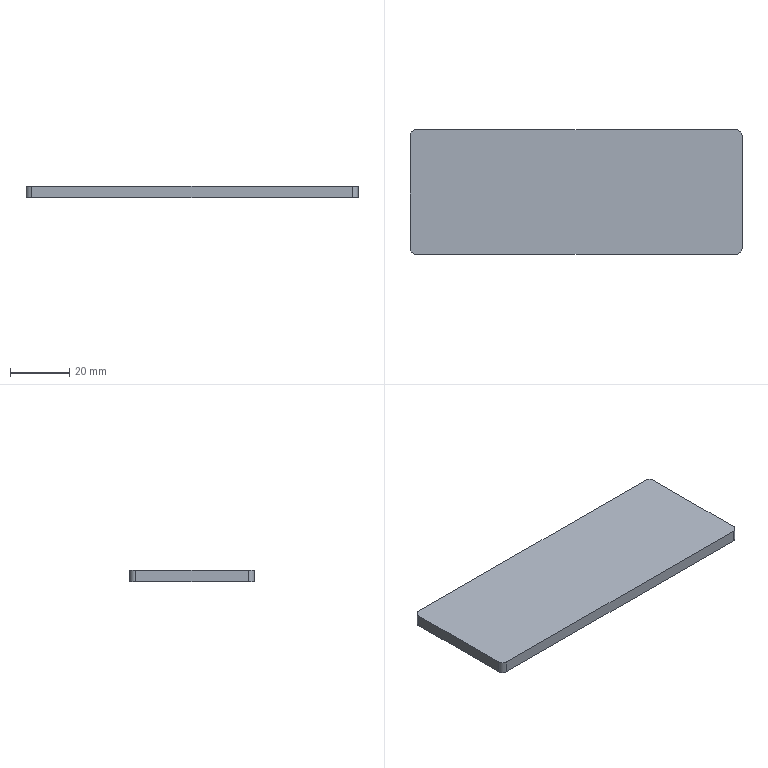Part | SolidWorks | features Extrusion 1 | 1 solid | 10 faces | box 112 x 42 x 4 mm | volume 18802 mm3 | plane 6 | cylinder 4 | commonest cylinder face diameters 4 x4
STEP:
#1=CARTESIAN_POINT('',(-54.,21.,0.));
#2=VERTEX_POINT('',#1);
#3=CARTESIAN_POINT('',(-56.,19.,0.));
#4=VERTEX_POINT('',#3);
#5=CARTESIAN_POINT('',(-54.,19.,0.));
#6=DIRECTION('',(0.,0.,1.));
#7=DIRECTION('',(1.,0.,0.));
#8=AXIS2_PLACEMENT_3D('',#5,#6,#7);
#9=CIRCLE('',#8,2.);
#10=EDGE_CURVE('',#2,#4,#9,.T.);
#11=ORIENTED_EDGE('',*,*,#10,.T.);
#12=CARTESIAN_POINT('',(-56.,19.,4.));
#13=VERTEX_POINT('',#12);
#14=CARTESIAN_POINT('',(-56.,19.,4.));
#15=DIRECTION('',(0.,0.,-1.));
#16=VECTOR('',#15,1000.);
#17=LINE('',#14,#16);
#18=EDGE_CURVE('',#13,#4,#17,.T.);
#19=ORIENTED_EDGE('',*,*,#18,.F.);
#20=CARTESIAN_POINT('',(-54.,21.,4.));
#21=VERTEX_POINT('',#20);
#22=CARTESIAN_POINT('',(-54.,19.,4.));
#23=DIRECTION('',(0.,0.,1.));
#24=DIRECTION('',(1.,0.,0.));
#25=AXIS2_PLACEMENT_3D('',#22,#23,#24);
#26=CIRCLE('',#25,2.);
#27=EDGE_CURVE('',#21,#13,#26,.T.);
#28=ORIENTED_EDGE('',*,*,#27,.F.);
#29=CARTESIAN_POINT('',(-54.,21.,4.));
#30=DIRECTION('',(0.,0.,-1.));
#31=VECTOR('',#30,1000.);
#32=LINE('',#29,#31);
#33=EDGE_CURVE('',#21,#2,#32,.T.);
#34=ORIENTED_EDGE('',*,*,#33,.T.);
#35=EDGE_LOOP('',(#11,#19,#28,#34));
#36=FACE_OUTER_BOUND('',#35,.T.);
#37=CARTESIAN_POINT('',(-54.,19.,4.));
#38=DIRECTION('',(0.,0.,-1.));
#39=DIRECTION('',(-1.,0.,0.));
#40=AXIS2_PLACEMENT_3D('',#37,#38,#39);
#41=CYLINDRICAL_SURFACE('',#40,2.);
#42=ADVANCED_FACE('',(#36),#41,.T.);
#43=CARTESIAN_POINT('',(-56.,-19.,0.));
#44=VERTEX_POINT('',#43);
#45=CARTESIAN_POINT('',(-56.,19.,0.));
#46=DIRECTION('',(0.,-1.,0.));
#47=VECTOR('',#46,1000.);
#48=LINE('',#45,#47);
#49=EDGE_CURVE('',#4,#44,#48,.T.);
#50=ORIENTED_EDGE('',*,*,#49,.T.);
#51=CARTESIAN_POINT('',(-56.,-19.,4.));
#52=VERTEX_POINT('',#51);
#53=CARTESIAN_POINT('',(-56.,-19.,4.));
#54=DIRECTION('',(0.,0.,-1.));
#55=VECTOR('',#54,1000.);
#56=LINE('',#53,#55);
#57=EDGE_CURVE('',#52,#44,#56,.T.);
#58=ORIENTED_EDGE('',*,*,#57,.F.);
#59=CARTESIAN_POINT('',(-56.,19.,4.));
#60=DIRECTION('',(0.,-1.,0.));
#61=VECTOR('',#60,1000.);
#62=LINE('',#59,#61);
#63=EDGE_CURVE('',#13,#52,#62,.T.);
#64=ORIENTED_EDGE('',*,*,#63,.F.);
#65=ORIENTED_EDGE('',*,*,#18,.T.);
#66=EDGE_LOOP('',(#50,#58,#64,#65));
#67=FACE_OUTER_BOUND('',#66,.T.);
#68=CARTESIAN_POINT('',(-56.,19.,4.));
#69=DIRECTION('',(1.,0.,0.));
#70=DIRECTION('',(0.,0.,-1.));
#71=AXIS2_PLACEMENT_3D('',#68,#69,#70);
#72=PLANE('',#71);
#73=ADVANCED_FACE('',(#67),#72,.F.);
#74=CARTESIAN_POINT('',(-54.,-21.,0.));
#75=VERTEX_POINT('',#74);
#76=CARTESIAN_POINT('',(-54.,-19.,0.));
#77=DIRECTION('',(0.,0.,-1.));
#78=DIRECTION('',(-1.,0.,0.));
#79=AXIS2_PLACEMENT_3D('',#76,#77,#78);
#80=CIRCLE('',#79,2.);
#81=EDGE_CURVE('',#75,#44,#80,.T.);
#82=ORIENTED_EDGE('',*,*,#81,.F.);
#83=CARTESIAN_POINT('',(-54.,-21.,4.));
#84=VERTEX_POINT('',#83);
#85=CARTESIAN_POINT('',(-54.,-21.,4.));
#86=DIRECTION('',(0.,0.,-1.));
#87=VECTOR('',#86,1000.);
#88=LINE('',#85,#87);
#89=EDGE_CURVE('',#84,#75,#88,.T.);
#90=ORIENTED_EDGE('',*,*,#89,.F.);
#91=CARTESIAN_POINT('',(-54.,-19.,4.));
#92=DIRECTION('',(0.,0.,-1.));
#93=DIRECTION('',(-1.,0.,0.));
#94=AXIS2_PLACEMENT_3D('',#91,#92,#93);
#95=CIRCLE('',#94,2.);
#96=EDGE_CURVE('',#84,#52,#95,.T.);
#97=ORIENTED_EDGE('',*,*,#96,.T.);
#98=ORIENTED_EDGE('',*,*,#57,.T.);
#99=EDGE_LOOP('',(#82,#90,#97,#98));
#100=FACE_OUTER_BOUND('',#99,.T.);
#101=CARTESIAN_POINT('',(-54.,-19.,4.));
#102=DIRECTION('',(0.,0.,-1.));
#103=DIRECTION('',(-1.,0.,0.));
#104=AXIS2_PLACEMENT_3D('',#101,#102,#103);
#105=CYLINDRICAL_SURFACE('',#104,2.);
#106=ADVANCED_FACE('',(#100),#105,.T.);
#107=CARTESIAN_POINT('',(54.,-21.,0.));
#108=VERTEX_POINT('',#107);
#109=CARTESIAN_POINT('',(54.,-21.,0.));
#110=DIRECTION('',(-1.,0.,0.));
#111=VECTOR('',#110,1000.);
#112=LINE('',#109,#111);
#113=EDGE_CURVE('',#108,#75,#112,.T.);
#114=ORIENTED_EDGE('',*,*,#113,.F.);
#115=CARTESIAN_POINT('',(54.,-21.,4.));
#116=VERTEX_POINT('',#115);
#117=CARTESIAN_POINT('',(54.,-21.,4.));
#118=DIRECTION('',(0.,0.,-1.));
#119=VECTOR('',#118,1000.);
#120=LINE('',#117,#119);
#121=EDGE_CURVE('',#116,#108,#120,.T.);
#122=ORIENTED_EDGE('',*,*,#121,.F.);
#123=CARTESIAN_POINT('',(54.,-21.,4.));
#124=DIRECTION('',(-1.,0.,0.));
#125=VECTOR('',#124,1000.);
#126=LINE('',#123,#125);
#127=EDGE_CURVE('',#116,#84,#126,.T.);
#128=ORIENTED_EDGE('',*,*,#127,.T.);
#129=ORIENTED_EDGE('',*,*,#89,.T.);
#130=EDGE_LOOP('',(#114,#122,#128,#129));
#131=FACE_OUTER_BOUND('',#130,.T.);
#132=CARTESIAN_POINT('',(54.,-21.,4.));
#133=DIRECTION('',(0.,-1.,0.));
#134=DIRECTION('',(1.,0.,0.));
#135=AXIS2_PLACEMENT_3D('',#132,#133,#134);
#136=PLANE('',#135);
#137=ADVANCED_FACE('',(#131),#136,.T.);
#138=CARTESIAN_POINT('',(56.,-19.,0.));
#139=VERTEX_POINT('',#138);
#140=CARTESIAN_POINT('',(54.,-19.,0.));
#141=DIRECTION('',(0.,0.,-1.));
#142=DIRECTION('',(-1.,0.,0.));
#143=AXIS2_PLACEMENT_3D('',#140,#141,#142);
#144=CIRCLE('',#143,2.);
#145=EDGE_CURVE('',#139,#108,#144,.T.);
#146=ORIENTED_EDGE('',*,*,#145,.F.);
#147=CARTESIAN_POINT('',(56.,-19.,4.));
#148=VERTEX_POINT('',#147);
#149=CARTESIAN_POINT('',(56.,-19.,4.));
#150=DIRECTION('',(0.,0.,-1.));
#151=VECTOR('',#150,1000.);
#152=LINE('',#149,#151);
#153=EDGE_CURVE('',#148,#139,#152,.T.);
#154=ORIENTED_EDGE('',*,*,#153,.F.);
#155=CARTESIAN_POINT('',(54.,-19.,4.));
#156=DIRECTION('',(0.,0.,-1.));
#157=DIRECTION('',(-1.,0.,0.));
#158=AXIS2_PLACEMENT_3D('',#155,#156,#157);
#159=CIRCLE('',#158,2.);
#160=EDGE_CURVE('',#148,#116,#159,.T.);
#161=ORIENTED_EDGE('',*,*,#160,.T.);
#162=ORIENTED_EDGE('',*,*,#121,.T.);
#163=EDGE_LOOP('',(#146,#154,#161,#162));
#164=FACE_OUTER_BOUND('',#163,.T.);
#165=CARTESIAN_POINT('',(54.,-19.,4.));
#166=DIRECTION('',(0.,0.,-1.));
#167=DIRECTION('',(-1.,0.,0.));
#168=AXIS2_PLACEMENT_3D('',#165,#166,#167);
#169=CYLINDRICAL_SURFACE('',#168,2.);
#170=ADVANCED_FACE('',(#164),#169,.T.);
#171=CARTESIAN_POINT('',(56.,19.,0.));
#172=VERTEX_POINT('',#171);
#173=CARTESIAN_POINT('',(56.,19.,0.));
#174=DIRECTION('',(0.,-1.,0.));
#175=VECTOR('',#174,1000.);
#176=LINE('',#173,#175);
#177=EDGE_CURVE('',#172,#139,#176,.T.);
#178=ORIENTED_EDGE('',*,*,#177,.F.);
#179=CARTESIAN_POINT('',(56.,19.,4.));
#180=VERTEX_POINT('',#179);
#181=CARTESIAN_POINT('',(56.,19.,4.));
#182=DIRECTION('',(0.,0.,-1.));
#183=VECTOR('',#182,1000.);
#184=LINE('',#181,#183);
#185=EDGE_CURVE('',#180,#172,#184,.T.);
#186=ORIENTED_EDGE('',*,*,#185,.F.);
#187=CARTESIAN_POINT('',(56.,19.,4.));
#188=DIRECTION('',(0.,-1.,0.));
#189=VECTOR('',#188,1000.);
#190=LINE('',#187,#189);
#191=EDGE_CURVE('',#180,#148,#190,.T.);
#192=ORIENTED_EDGE('',*,*,#191,.T.);
#193=ORIENTED_EDGE('',*,*,#153,.T.);
#194=EDGE_LOOP('',(#178,#186,#192,#193));
#195=FACE_OUTER_BOUND('',#194,.T.);
#196=CARTESIAN_POINT('',(56.,19.,4.));
#197=DIRECTION('',(1.,0.,0.));
#198=DIRECTION('',(0.,1.,0.));
#199=AXIS2_PLACEMENT_3D('',#196,#197,#198);
#200=PLANE('',#199);
#201=ADVANCED_FACE('',(#195),#200,.T.);
#202=CARTESIAN_POINT('',(54.,21.,0.));
#203=VERTEX_POINT('',#202);
#204=CARTESIAN_POINT('',(54.,19.,0.));
#205=DIRECTION('',(0.,0.,-1.));
#206=DIRECTION('',(-1.,0.,0.));
#207=AXIS2_PLACEMENT_3D('',#204,#205,#206);
#208=CIRCLE('',#207,2.);
#209=EDGE_CURVE('',#203,#172,#208,.T.);
#210=ORIENTED_EDGE('',*,*,#209,.F.);
#211=CARTESIAN_POINT('',(54.,21.,4.));
#212=VERTEX_POINT('',#211);
#213=CARTESIAN_POINT('',(54.,21.,4.));
#214=DIRECTION('',(0.,0.,-1.));
#215=VECTOR('',#214,1000.);
#216=LINE('',#213,#215);
#217=EDGE_CURVE('',#212,#203,#216,.T.);
#218=ORIENTED_EDGE('',*,*,#217,.F.);
#219=CARTESIAN_POINT('',(54.,19.,4.));
#220=DIRECTION('',(0.,0.,-1.));
#221=DIRECTION('',(-1.,0.,0.));
#222=AXIS2_PLACEMENT_3D('',#219,#220,#221);
#223=CIRCLE('',#222,2.);
#224=EDGE_CURVE('',#212,#180,#223,.T.);
#225=ORIENTED_EDGE('',*,*,#224,.T.);
#226=ORIENTED_EDGE('',*,*,#185,.T.);
#227=EDGE_LOOP('',(#210,#218,#225,#226));
#228=FACE_OUTER_BOUND('',#227,.T.);
#229=CARTESIAN_POINT('',(54.,19.,4.));
#230=DIRECTION('',(0.,0.,-1.));
#231=DIRECTION('',(-1.,0.,0.));
#232=AXIS2_PLACEMENT_3D('',#229,#230,#231);
#233=CYLINDRICAL_SURFACE('',#232,2.);
#234=ADVANCED_FACE('',(#228),#233,.T.);
#235=CARTESIAN_POINT('',(54.,21.,0.));
#236=DIRECTION('',(-1.,0.,0.));
#237=VECTOR('',#236,1000.);
#238=LINE('',#235,#237);
#239=EDGE_CURVE('',#203,#2,#238,.T.);
#240=ORIENTED_EDGE('',*,*,#239,.T.);
#241=ORIENTED_EDGE('',*,*,#33,.F.);
#242=CARTESIAN_POINT('',(54.,21.,4.));
#243=DIRECTION('',(-1.,0.,0.));
#244=VECTOR('',#243,1000.);
#245=LINE('',#242,#244);
#246=EDGE_CURVE('',#212,#21,#245,.T.);
#247=ORIENTED_EDGE('',*,*,#246,.F.);
#248=ORIENTED_EDGE('',*,*,#217,.T.);
#249=EDGE_LOOP('',(#240,#241,#247,#248));
#250=FACE_OUTER_BOUND('',#249,.T.);
#251=CARTESIAN_POINT('',(54.,21.,4.));
#252=DIRECTION('',(0.,-1.,0.));
#253=DIRECTION('',(1.,0.,0.));
#254=AXIS2_PLACEMENT_3D('',#251,#252,#253);
#255=PLANE('',#254);
#256=ADVANCED_FACE('',(#250),#255,.F.);
#257=ORIENTED_EDGE('',*,*,#27,.T.);
#258=ORIENTED_EDGE('',*,*,#63,.T.);
#259=ORIENTED_EDGE('',*,*,#96,.F.);
#260=ORIENTED_EDGE('',*,*,#127,.F.);
#261=ORIENTED_EDGE('',*,*,#160,.F.);
#262=ORIENTED_EDGE('',*,*,#191,.F.);
#263=ORIENTED_EDGE('',*,*,#224,.F.);
#264=ORIENTED_EDGE('',*,*,#246,.T.);
#265=EDGE_LOOP('',(#257,#258,#259,#260,#261,#262,#263,#264));
#266=FACE_OUTER_BOUND('',#265,.T.);
#267=CARTESIAN_POINT('',(-54.,19.,4.));
#268=DIRECTION('',(0.,0.,1.));
#269=DIRECTION('',(1.,0.,0.));
#270=AXIS2_PLACEMENT_3D('',#267,#268,#269);
#271=PLANE('',#270);
#272=ADVANCED_FACE('',(#266),#271,.T.);
#273=ORIENTED_EDGE('',*,*,#10,.F.);
#274=ORIENTED_EDGE('',*,*,#239,.F.);
#275=ORIENTED_EDGE('',*,*,#209,.T.);
#276=ORIENTED_EDGE('',*,*,#177,.T.);
#277=ORIENTED_EDGE('',*,*,#145,.T.);
#278=ORIENTED_EDGE('',*,*,#113,.T.);
#279=ORIENTED_EDGE('',*,*,#81,.T.);
#280=ORIENTED_EDGE('',*,*,#49,.F.);
#281=EDGE_LOOP('',(#273,#274,#275,#276,#277,#278,#279,#280));
#282=FACE_OUTER_BOUND('',#281,.T.);
#283=CARTESIAN_POINT('',(-54.,19.,0.));
#284=DIRECTION('',(0.,0.,1.));
#285=DIRECTION('',(1.,0.,0.));
#286=AXIS2_PLACEMENT_3D('',#283,#284,#285);
#287=PLANE('',#286);
#288=ADVANCED_FACE('',(#282),#287,.F.);
#289=CLOSED_SHELL('',(#42,#73,#106,#137,#170,#201,#234,#256,#272,#288));
#290=MANIFOLD_SOLID_BREP('',#289);
#291=CARTESIAN_POINT('',(0.,0.,0.));
#292=DIRECTION('',(0.,0.,1.));
#293=DIRECTION('',(1.,0.,0.));
#294=AXIS2_PLACEMENT_3D('',#291,#292,#293);
#295=(LENGTH_UNIT()NAMED_UNIT(*)SI_UNIT(.MILLI.,.METRE.));
#296=UNCERTAINTY_MEASURE_WITH_UNIT(LENGTH_MEASURE(0.00001),#295,'','');
#297=(NAMED_UNIT(*)PLANE_ANGLE_UNIT()SI_UNIT($,.RADIAN.));
#298=(NAMED_UNIT(*)SI_UNIT($,.STERADIAN.)SOLID_ANGLE_UNIT());
#299=(GEOMETRIC_REPRESENTATION_CONTEXT(3)GLOBAL_UNCERTAINTY_ASSIGNED_CONTEXT((#296))GLOBAL_UNIT_ASSIGNED_CONTEXT((#295,#297,#298))REPRESENTATION_CONTEXT('',''));
#300=ADVANCED_BREP_SHAPE_REPRESENTATION('',(#290,#294),#299);